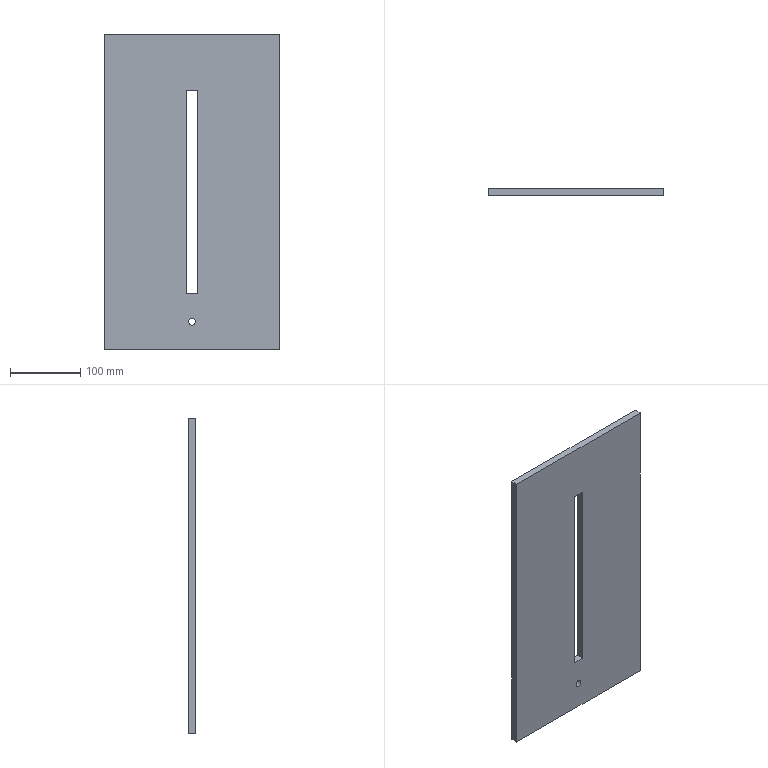Part | STEP file | tieqianjijia | 1 solid | 11 faces | box 250 x 10 x 450 mm | volume 1077815 mm3 | plane 10 | cylinder 1 | commonest cylinder face diameters 10 x1
STEP:
#1=CARTESIAN_POINT('',(0.,0.,0.));
#2=DIRECTION('',(0.,0.,1.));
#3=DIRECTION('',(1.,0.,0.));
#4=AXIS2_PLACEMENT_3D('',#1,#2,#3);
#5=CARTESIAN_POINT('',(0.,5.,-180.));
#6=VERTEX_POINT('',#5);
#7=CARTESIAN_POINT('',(0.,5.,-185.));
#8=DIRECTION('',(0.,1.,0.));
#9=DIRECTION('',(0.,0.,1.));
#10=AXIS2_PLACEMENT_3D('',#7,#8,#9);
#11=CIRCLE('',#10,5.);
#12=CARTESIAN_POINT('',(0.,5.,0.));
#13=DIRECTION('',(0.,1.,0.));
#14=DIRECTION('',(0.,0.,1.));
#15=AXIS2_PLACEMENT_3D('',#12,#13,#14);
#16=PLANE('',#15);
#17=CARTESIAN_POINT('',(-185.,0.));
#18=DIRECTION('',(1.,0.));
#19=AXIS2_PLACEMENT_2D('',#17,#18);
#20=CIRCLE('',#19,5.);
#21=(GEOMETRIC_REPRESENTATION_CONTEXT(2)PARAMETRIC_REPRESENTATION_CONTEXT()REPRESENTATION_CONTEXT('',''));
#22=DEFINITIONAL_REPRESENTATION('',(#20),#21);
#23=PCURVE('',#16,#22);
#24=CARTESIAN_POINT('',(0.,-5.,-185.));
#25=DIRECTION('',(0.,1.,0.));
#26=DIRECTION('',(0.,0.,1.));
#27=AXIS2_PLACEMENT_3D('',#24,#25,#26);
#28=CYLINDRICAL_SURFACE('',#27,5.);
#29=CARTESIAN_POINT('',(0.,10.));
#30=DIRECTION('',(1.,0.));
#31=VECTOR('',#30,1.);
#32=LINE('',#29,#31);
#33=(GEOMETRIC_REPRESENTATION_CONTEXT(2)PARAMETRIC_REPRESENTATION_CONTEXT()REPRESENTATION_CONTEXT('',''));
#34=DEFINITIONAL_REPRESENTATION('',(#32),#33);
#35=PCURVE('',#28,#34);
#36=SURFACE_CURVE('',#11,(#23,#35),.PCURVE_S1.);
#37=EDGE_CURVE('',#6,#6,#36,.T.);
#38=ORIENTED_EDGE('',*,*,#37,.F.);
#39=EDGE_LOOP('',(#38));
#40=FACE_BOUND('',#39,.T.);
#41=CARTESIAN_POINT('',(125.,5.,225.));
#42=VERTEX_POINT('',#41);
#43=CARTESIAN_POINT('',(125.,5.,-225.));
#44=VERTEX_POINT('',#43);
#45=CARTESIAN_POINT('',(125.,5.,-225.));
#46=DIRECTION('',(0.,0.,-1.));
#47=VECTOR('',#46,1.);
#48=LINE('',#45,#47);
#49=CARTESIAN_POINT('',(-225.,125.));
#50=DIRECTION('',(-1.,0.));
#51=VECTOR('',#50,1.);
#52=LINE('',#49,#51);
#53=(GEOMETRIC_REPRESENTATION_CONTEXT(2)PARAMETRIC_REPRESENTATION_CONTEXT()REPRESENTATION_CONTEXT('',''));
#54=DEFINITIONAL_REPRESENTATION('',(#52),#53);
#55=PCURVE('',#16,#54);
#56=CARTESIAN_POINT('',(125.,5.,-225.));
#57=DIRECTION('',(-1.,0.,0.));
#58=DIRECTION('',(0.,0.,1.));
#59=AXIS2_PLACEMENT_3D('',#56,#57,#58);
#60=PLANE('',#59);
#61=CARTESIAN_POINT('',(0.,0.));
#62=DIRECTION('',(-1.,0.));
#63=VECTOR('',#62,1.);
#64=LINE('',#61,#63);
#65=(GEOMETRIC_REPRESENTATION_CONTEXT(2)PARAMETRIC_REPRESENTATION_CONTEXT()REPRESENTATION_CONTEXT('',''));
#66=DEFINITIONAL_REPRESENTATION('',(#64),#65);
#67=PCURVE('',#60,#66);
#68=SURFACE_CURVE('',#48,(#55,#67),.PCURVE_S1.);
#69=EDGE_CURVE('',#42,#44,#68,.T.);
#70=ORIENTED_EDGE('',*,*,#69,.T.);
#71=CARTESIAN_POINT('',(-125.,5.,-225.));
#72=VERTEX_POINT('',#71);
#73=CARTESIAN_POINT('',(-125.,5.,-225.));
#74=DIRECTION('',(-1.,0.,0.));
#75=VECTOR('',#74,1.);
#76=LINE('',#73,#75);
#77=CARTESIAN_POINT('',(-225.,-125.));
#78=DIRECTION('',(0.,-1.));
#79=VECTOR('',#78,1.);
#80=LINE('',#77,#79);
#81=(GEOMETRIC_REPRESENTATION_CONTEXT(2)PARAMETRIC_REPRESENTATION_CONTEXT()REPRESENTATION_CONTEXT('',''));
#82=DEFINITIONAL_REPRESENTATION('',(#80),#81);
#83=PCURVE('',#16,#82);
#84=CARTESIAN_POINT('',(-125.,5.,-225.));
#85=DIRECTION('',(0.,0.,1.));
#86=DIRECTION('',(1.,0.,0.));
#87=AXIS2_PLACEMENT_3D('',#84,#85,#86);
#88=PLANE('',#87);
#89=CARTESIAN_POINT('',(0.,0.));
#90=DIRECTION('',(-1.,0.));
#91=VECTOR('',#90,1.);
#92=LINE('',#89,#91);
#93=(GEOMETRIC_REPRESENTATION_CONTEXT(2)PARAMETRIC_REPRESENTATION_CONTEXT()REPRESENTATION_CONTEXT('',''));
#94=DEFINITIONAL_REPRESENTATION('',(#92),#93);
#95=PCURVE('',#88,#94);
#96=SURFACE_CURVE('',#76,(#83,#95),.PCURVE_S1.);
#97=EDGE_CURVE('',#44,#72,#96,.T.);
#98=ORIENTED_EDGE('',*,*,#97,.T.);
#99=CARTESIAN_POINT('',(-125.,5.,225.));
#100=VERTEX_POINT('',#99);
#101=CARTESIAN_POINT('',(-125.,5.,-225.));
#102=DIRECTION('',(0.,0.,1.));
#103=VECTOR('',#102,1.);
#104=LINE('',#101,#103);
#105=CARTESIAN_POINT('',(-225.,-125.));
#106=DIRECTION('',(1.,0.));
#107=VECTOR('',#106,1.);
#108=LINE('',#105,#107);
#109=(GEOMETRIC_REPRESENTATION_CONTEXT(2)PARAMETRIC_REPRESENTATION_CONTEXT()REPRESENTATION_CONTEXT('',''));
#110=DEFINITIONAL_REPRESENTATION('',(#108),#109);
#111=PCURVE('',#16,#110);
#112=CARTESIAN_POINT('',(-125.,5.,-225.));
#113=DIRECTION('',(1.,0.,0.));
#114=DIRECTION('',(0.,0.,-1.));
#115=AXIS2_PLACEMENT_3D('',#112,#113,#114);
#116=PLANE('',#115);
#117=CARTESIAN_POINT('',(0.,0.));
#118=DIRECTION('',(-1.,0.));
#119=VECTOR('',#118,1.);
#120=LINE('',#117,#119);
#121=(GEOMETRIC_REPRESENTATION_CONTEXT(2)PARAMETRIC_REPRESENTATION_CONTEXT()REPRESENTATION_CONTEXT('',''));
#122=DEFINITIONAL_REPRESENTATION('',(#120),#121);
#123=PCURVE('',#116,#122);
#124=SURFACE_CURVE('',#104,(#111,#123),.PCURVE_S1.);
#125=EDGE_CURVE('',#72,#100,#124,.T.);
#126=ORIENTED_EDGE('',*,*,#125,.T.);
#127=CARTESIAN_POINT('',(-125.,5.,225.));
#128=DIRECTION('',(1.,0.,0.));
#129=VECTOR('',#128,1.);
#130=LINE('',#127,#129);
#131=CARTESIAN_POINT('',(225.,-125.));
#132=DIRECTION('',(0.,1.));
#133=VECTOR('',#132,1.);
#134=LINE('',#131,#133);
#135=(GEOMETRIC_REPRESENTATION_CONTEXT(2)PARAMETRIC_REPRESENTATION_CONTEXT()REPRESENTATION_CONTEXT('',''));
#136=DEFINITIONAL_REPRESENTATION('',(#134),#135);
#137=PCURVE('',#16,#136);
#138=CARTESIAN_POINT('',(-125.,5.,225.));
#139=DIRECTION('',(0.,0.,-1.));
#140=DIRECTION('',(-1.,0.,0.));
#141=AXIS2_PLACEMENT_3D('',#138,#139,#140);
#142=PLANE('',#141);
#143=CARTESIAN_POINT('',(0.,0.));
#144=DIRECTION('',(-1.,0.));
#145=VECTOR('',#144,1.);
#146=LINE('',#143,#145);
#147=(GEOMETRIC_REPRESENTATION_CONTEXT(2)PARAMETRIC_REPRESENTATION_CONTEXT()REPRESENTATION_CONTEXT('',''));
#148=DEFINITIONAL_REPRESENTATION('',(#146),#147);
#149=PCURVE('',#142,#148);
#150=SURFACE_CURVE('',#130,(#137,#149),.PCURVE_S1.);
#151=EDGE_CURVE('',#100,#42,#150,.T.);
#152=ORIENTED_EDGE('',*,*,#151,.T.);
#153=EDGE_LOOP('',(#70,#98,#126,#152));
#154=FACE_BOUND('',#153,.T.);
#155=CARTESIAN_POINT('',(8.,5.,-145.));
#156=VERTEX_POINT('',#155);
#157=CARTESIAN_POINT('',(-8.,5.,-145.));
#158=VERTEX_POINT('',#157);
#159=CARTESIAN_POINT('',(-8.,5.,-145.));
#160=DIRECTION('',(-1.,0.,0.));
#161=VECTOR('',#160,1.);
#162=LINE('',#159,#161);
#163=CARTESIAN_POINT('',(-145.,-8.));
#164=DIRECTION('',(0.,-1.));
#165=VECTOR('',#164,1.);
#166=LINE('',#163,#165);
#167=(GEOMETRIC_REPRESENTATION_CONTEXT(2)PARAMETRIC_REPRESENTATION_CONTEXT()REPRESENTATION_CONTEXT('',''));
#168=DEFINITIONAL_REPRESENTATION('',(#166),#167);
#169=PCURVE('',#16,#168);
#170=CARTESIAN_POINT('',(-8.,5.,-145.));
#171=DIRECTION('',(0.,0.,1.));
#172=DIRECTION('',(1.,0.,0.));
#173=AXIS2_PLACEMENT_3D('',#170,#171,#172);
#174=PLANE('',#173);
#175=CARTESIAN_POINT('',(0.,0.));
#176=DIRECTION('',(-1.,0.));
#177=VECTOR('',#176,1.);
#178=LINE('',#175,#177);
#179=(GEOMETRIC_REPRESENTATION_CONTEXT(2)PARAMETRIC_REPRESENTATION_CONTEXT()REPRESENTATION_CONTEXT('',''));
#180=DEFINITIONAL_REPRESENTATION('',(#178),#179);
#181=PCURVE('',#174,#180);
#182=SURFACE_CURVE('',#162,(#169,#181),.PCURVE_S1.);
#183=EDGE_CURVE('',#156,#158,#182,.T.);
#184=ORIENTED_EDGE('',*,*,#183,.F.);
#185=CARTESIAN_POINT('',(8.,5.,145.));
#186=VERTEX_POINT('',#185);
#187=CARTESIAN_POINT('',(8.,5.,-145.));
#188=DIRECTION('',(0.,0.,-1.));
#189=VECTOR('',#188,1.);
#190=LINE('',#187,#189);
#191=CARTESIAN_POINT('',(-145.,8.));
#192=DIRECTION('',(-1.,0.));
#193=VECTOR('',#192,1.);
#194=LINE('',#191,#193);
#195=(GEOMETRIC_REPRESENTATION_CONTEXT(2)PARAMETRIC_REPRESENTATION_CONTEXT()REPRESENTATION_CONTEXT('',''));
#196=DEFINITIONAL_REPRESENTATION('',(#194),#195);
#197=PCURVE('',#16,#196);
#198=CARTESIAN_POINT('',(8.,5.,-145.));
#199=DIRECTION('',(-1.,0.,0.));
#200=DIRECTION('',(0.,0.,1.));
#201=AXIS2_PLACEMENT_3D('',#198,#199,#200);
#202=PLANE('',#201);
#203=CARTESIAN_POINT('',(0.,0.));
#204=DIRECTION('',(-1.,0.));
#205=VECTOR('',#204,1.);
#206=LINE('',#203,#205);
#207=(GEOMETRIC_REPRESENTATION_CONTEXT(2)PARAMETRIC_REPRESENTATION_CONTEXT()REPRESENTATION_CONTEXT('',''));
#208=DEFINITIONAL_REPRESENTATION('',(#206),#207);
#209=PCURVE('',#202,#208);
#210=SURFACE_CURVE('',#190,(#197,#209),.PCURVE_S1.);
#211=EDGE_CURVE('',#186,#156,#210,.T.);
#212=ORIENTED_EDGE('',*,*,#211,.F.);
#213=CARTESIAN_POINT('',(-8.,5.,145.));
#214=VERTEX_POINT('',#213);
#215=CARTESIAN_POINT('',(-8.,5.,145.));
#216=DIRECTION('',(1.,0.,0.));
#217=VECTOR('',#216,1.);
#218=LINE('',#215,#217);
#219=CARTESIAN_POINT('',(145.,-8.));
#220=DIRECTION('',(0.,1.));
#221=VECTOR('',#220,1.);
#222=LINE('',#219,#221);
#223=(GEOMETRIC_REPRESENTATION_CONTEXT(2)PARAMETRIC_REPRESENTATION_CONTEXT()REPRESENTATION_CONTEXT('',''));
#224=DEFINITIONAL_REPRESENTATION('',(#222),#223);
#225=PCURVE('',#16,#224);
#226=CARTESIAN_POINT('',(-8.,5.,145.));
#227=DIRECTION('',(0.,0.,-1.));
#228=DIRECTION('',(-1.,0.,0.));
#229=AXIS2_PLACEMENT_3D('',#226,#227,#228);
#230=PLANE('',#229);
#231=CARTESIAN_POINT('',(0.,0.));
#232=DIRECTION('',(-1.,0.));
#233=VECTOR('',#232,1.);
#234=LINE('',#231,#233);
#235=(GEOMETRIC_REPRESENTATION_CONTEXT(2)PARAMETRIC_REPRESENTATION_CONTEXT()REPRESENTATION_CONTEXT('',''));
#236=DEFINITIONAL_REPRESENTATION('',(#234),#235);
#237=PCURVE('',#230,#236);
#238=SURFACE_CURVE('',#218,(#225,#237),.PCURVE_S1.);
#239=EDGE_CURVE('',#214,#186,#238,.T.);
#240=ORIENTED_EDGE('',*,*,#239,.F.);
#241=CARTESIAN_POINT('',(-8.,5.,-145.));
#242=DIRECTION('',(0.,0.,1.));
#243=VECTOR('',#242,1.);
#244=LINE('',#241,#243);
#245=CARTESIAN_POINT('',(-145.,-8.));
#246=DIRECTION('',(1.,0.));
#247=VECTOR('',#246,1.);
#248=LINE('',#245,#247);
#249=(GEOMETRIC_REPRESENTATION_CONTEXT(2)PARAMETRIC_REPRESENTATION_CONTEXT()REPRESENTATION_CONTEXT('',''));
#250=DEFINITIONAL_REPRESENTATION('',(#248),#249);
#251=PCURVE('',#16,#250);
#252=CARTESIAN_POINT('',(-8.,5.,-145.));
#253=DIRECTION('',(1.,0.,0.));
#254=DIRECTION('',(0.,0.,-1.));
#255=AXIS2_PLACEMENT_3D('',#252,#253,#254);
#256=PLANE('',#255);
#257=CARTESIAN_POINT('',(0.,0.));
#258=DIRECTION('',(-1.,0.));
#259=VECTOR('',#258,1.);
#260=LINE('',#257,#259);
#261=(GEOMETRIC_REPRESENTATION_CONTEXT(2)PARAMETRIC_REPRESENTATION_CONTEXT()REPRESENTATION_CONTEXT('',''));
#262=DEFINITIONAL_REPRESENTATION('',(#260),#261);
#263=PCURVE('',#256,#262);
#264=SURFACE_CURVE('',#244,(#251,#263),.PCURVE_S1.);
#265=EDGE_CURVE('',#158,#214,#264,.T.);
#266=ORIENTED_EDGE('',*,*,#265,.F.);
#267=EDGE_LOOP('',(#184,#212,#240,#266));
#268=FACE_BOUND('',#267,.T.);
#269=ADVANCED_FACE('',(#40,#154,#268),#16,.T.);
#270=CARTESIAN_POINT('',(0.,-5.,-180.));
#271=VERTEX_POINT('',#270);
#272=CARTESIAN_POINT('',(0.,-5.,-185.));
#273=DIRECTION('',(0.,1.,0.));
#274=DIRECTION('',(0.,0.,1.));
#275=AXIS2_PLACEMENT_3D('',#272,#273,#274);
#276=CIRCLE('',#275,5.);
#277=CARTESIAN_POINT('',(0.,-5.,0.));
#278=DIRECTION('',(0.,1.,0.));
#279=DIRECTION('',(0.,0.,1.));
#280=AXIS2_PLACEMENT_3D('',#277,#278,#279);
#281=PLANE('',#280);
#282=CARTESIAN_POINT('',(-185.,0.));
#283=DIRECTION('',(1.,0.));
#284=AXIS2_PLACEMENT_2D('',#282,#283);
#285=CIRCLE('',#284,5.);
#286=(GEOMETRIC_REPRESENTATION_CONTEXT(2)PARAMETRIC_REPRESENTATION_CONTEXT()REPRESENTATION_CONTEXT('',''));
#287=DEFINITIONAL_REPRESENTATION('',(#285),#286);
#288=PCURVE('',#281,#287);
#289=CARTESIAN_POINT('',(0.,0.));
#290=DIRECTION('',(1.,0.));
#291=VECTOR('',#290,1.);
#292=LINE('',#289,#291);
#293=(GEOMETRIC_REPRESENTATION_CONTEXT(2)PARAMETRIC_REPRESENTATION_CONTEXT()REPRESENTATION_CONTEXT('',''));
#294=DEFINITIONAL_REPRESENTATION('',(#292),#293);
#295=PCURVE('',#28,#294);
#296=SURFACE_CURVE('',#276,(#288,#295),.PCURVE_S1.);
#297=EDGE_CURVE('',#271,#271,#296,.T.);
#298=ORIENTED_EDGE('',*,*,#297,.T.);
#299=EDGE_LOOP('',(#298));
#300=FACE_BOUND('',#299,.T.);
#301=CARTESIAN_POINT('',(125.,-5.,225.));
#302=VERTEX_POINT('',#301);
#303=CARTESIAN_POINT('',(125.,-5.,-225.));
#304=VERTEX_POINT('',#303);
#305=CARTESIAN_POINT('',(125.,-5.,-225.));
#306=DIRECTION('',(0.,0.,-1.));
#307=VECTOR('',#306,1.);
#308=LINE('',#305,#307);
#309=CARTESIAN_POINT('',(-225.,125.));
#310=DIRECTION('',(-1.,0.));
#311=VECTOR('',#310,1.);
#312=LINE('',#309,#311);
#313=(GEOMETRIC_REPRESENTATION_CONTEXT(2)PARAMETRIC_REPRESENTATION_CONTEXT()REPRESENTATION_CONTEXT('',''));
#314=DEFINITIONAL_REPRESENTATION('',(#312),#313);
#315=PCURVE('',#281,#314);
#316=CARTESIAN_POINT('',(0.,-10.));
#317=DIRECTION('',(-1.,0.));
#318=VECTOR('',#317,1.);
#319=LINE('',#316,#318);
#320=(GEOMETRIC_REPRESENTATION_CONTEXT(2)PARAMETRIC_REPRESENTATION_CONTEXT()REPRESENTATION_CONTEXT('',''));
#321=DEFINITIONAL_REPRESENTATION('',(#319),#320);
#322=PCURVE('',#60,#321);
#323=SURFACE_CURVE('',#308,(#315,#322),.PCURVE_S1.);
#324=EDGE_CURVE('',#302,#304,#323,.T.);
#325=ORIENTED_EDGE('',*,*,#324,.F.);
#326=CARTESIAN_POINT('',(-125.,-5.,225.));
#327=VERTEX_POINT('',#326);
#328=CARTESIAN_POINT('',(-125.,-5.,225.));
#329=DIRECTION('',(1.,0.,0.));
#330=VECTOR('',#329,1.);
#331=LINE('',#328,#330);
#332=CARTESIAN_POINT('',(225.,-125.));
#333=DIRECTION('',(0.,1.));
#334=VECTOR('',#333,1.);
#335=LINE('',#332,#334);
#336=(GEOMETRIC_REPRESENTATION_CONTEXT(2)PARAMETRIC_REPRESENTATION_CONTEXT()REPRESENTATION_CONTEXT('',''));
#337=DEFINITIONAL_REPRESENTATION('',(#335),#336);
#338=PCURVE('',#281,#337);
#339=CARTESIAN_POINT('',(0.,-10.));
#340=DIRECTION('',(-1.,0.));
#341=VECTOR('',#340,1.);
#342=LINE('',#339,#341);
#343=(GEOMETRIC_REPRESENTATION_CONTEXT(2)PARAMETRIC_REPRESENTATION_CONTEXT()REPRESENTATION_CONTEXT('',''));
#344=DEFINITIONAL_REPRESENTATION('',(#342),#343);
#345=PCURVE('',#142,#344);
#346=SURFACE_CURVE('',#331,(#338,#345),.PCURVE_S1.);
#347=EDGE_CURVE('',#327,#302,#346,.T.);
#348=ORIENTED_EDGE('',*,*,#347,.F.);
#349=CARTESIAN_POINT('',(-125.,-5.,-225.));
#350=VERTEX_POINT('',#349);
#351=CARTESIAN_POINT('',(-125.,-5.,-225.));
#352=DIRECTION('',(0.,0.,1.));
#353=VECTOR('',#352,1.);
#354=LINE('',#351,#353);
#355=CARTESIAN_POINT('',(-225.,-125.));
#356=DIRECTION('',(1.,0.));
#357=VECTOR('',#356,1.);
#358=LINE('',#355,#357);
#359=(GEOMETRIC_REPRESENTATION_CONTEXT(2)PARAMETRIC_REPRESENTATION_CONTEXT()REPRESENTATION_CONTEXT('',''));
#360=DEFINITIONAL_REPRESENTATION('',(#358),#359);
#361=PCURVE('',#281,#360);
#362=CARTESIAN_POINT('',(0.,-10.));
#363=DIRECTION('',(-1.,0.));
#364=VECTOR('',#363,1.);
#365=LINE('',#362,#364);
#366=(GEOMETRIC_REPRESENTATION_CONTEXT(2)PARAMETRIC_REPRESENTATION_CONTEXT()REPRESENTATION_CONTEXT('',''));
#367=DEFINITIONAL_REPRESENTATION('',(#365),#366);
#368=PCURVE('',#116,#367);
#369=SURFACE_CURVE('',#354,(#361,#368),.PCURVE_S1.);
#370=EDGE_CURVE('',#350,#327,#369,.T.);
#371=ORIENTED_EDGE('',*,*,#370,.F.);
#372=CARTESIAN_POINT('',(-125.,-5.,-225.));
#373=DIRECTION('',(-1.,0.,0.));
#374=VECTOR('',#373,1.);
#375=LINE('',#372,#374);
#376=CARTESIAN_POINT('',(-225.,-125.));
#377=DIRECTION('',(0.,-1.));
#378=VECTOR('',#377,1.);
#379=LINE('',#376,#378);
#380=(GEOMETRIC_REPRESENTATION_CONTEXT(2)PARAMETRIC_REPRESENTATION_CONTEXT()REPRESENTATION_CONTEXT('',''));
#381=DEFINITIONAL_REPRESENTATION('',(#379),#380);
#382=PCURVE('',#281,#381);
#383=CARTESIAN_POINT('',(0.,-10.));
#384=DIRECTION('',(-1.,0.));
#385=VECTOR('',#384,1.);
#386=LINE('',#383,#385);
#387=(GEOMETRIC_REPRESENTATION_CONTEXT(2)PARAMETRIC_REPRESENTATION_CONTEXT()REPRESENTATION_CONTEXT('',''));
#388=DEFINITIONAL_REPRESENTATION('',(#386),#387);
#389=PCURVE('',#88,#388);
#390=SURFACE_CURVE('',#375,(#382,#389),.PCURVE_S1.);
#391=EDGE_CURVE('',#304,#350,#390,.T.);
#392=ORIENTED_EDGE('',*,*,#391,.F.);
#393=EDGE_LOOP('',(#325,#348,#371,#392));
#394=FACE_BOUND('',#393,.T.);
#395=CARTESIAN_POINT('',(8.,-5.,145.));
#396=VERTEX_POINT('',#395);
#397=CARTESIAN_POINT('',(8.,-5.,-145.));
#398=VERTEX_POINT('',#397);
#399=CARTESIAN_POINT('',(8.,-5.,-145.));
#400=DIRECTION('',(0.,0.,-1.));
#401=VECTOR('',#400,1.);
#402=LINE('',#399,#401);
#403=CARTESIAN_POINT('',(-145.,8.));
#404=DIRECTION('',(-1.,0.));
#405=VECTOR('',#404,1.);
#406=LINE('',#403,#405);
#407=(GEOMETRIC_REPRESENTATION_CONTEXT(2)PARAMETRIC_REPRESENTATION_CONTEXT()REPRESENTATION_CONTEXT('',''));
#408=DEFINITIONAL_REPRESENTATION('',(#406),#407);
#409=PCURVE('',#281,#408);
#410=CARTESIAN_POINT('',(0.,-10.));
#411=DIRECTION('',(-1.,0.));
#412=VECTOR('',#411,1.);
#413=LINE('',#410,#412);
#414=(GEOMETRIC_REPRESENTATION_CONTEXT(2)PARAMETRIC_REPRESENTATION_CONTEXT()REPRESENTATION_CONTEXT('',''));
#415=DEFINITIONAL_REPRESENTATION('',(#413),#414);
#416=PCURVE('',#202,#415);
#417=SURFACE_CURVE('',#402,(#409,#416),.PCURVE_S1.);
#418=EDGE_CURVE('',#396,#398,#417,.T.);
#419=ORIENTED_EDGE('',*,*,#418,.T.);
#420=CARTESIAN_POINT('',(-8.,-5.,-145.));
#421=VERTEX_POINT('',#420);
#422=CARTESIAN_POINT('',(-8.,-5.,-145.));
#423=DIRECTION('',(-1.,0.,0.));
#424=VECTOR('',#423,1.);
#425=LINE('',#422,#424);
#426=CARTESIAN_POINT('',(-145.,-8.));
#427=DIRECTION('',(0.,-1.));
#428=VECTOR('',#427,1.);
#429=LINE('',#426,#428);
#430=(GEOMETRIC_REPRESENTATION_CONTEXT(2)PARAMETRIC_REPRESENTATION_CONTEXT()REPRESENTATION_CONTEXT('',''));
#431=DEFINITIONAL_REPRESENTATION('',(#429),#430);
#432=PCURVE('',#281,#431);
#433=CARTESIAN_POINT('',(0.,-10.));
#434=DIRECTION('',(-1.,0.));
#435=VECTOR('',#434,1.);
#436=LINE('',#433,#435);
#437=(GEOMETRIC_REPRESENTATION_CONTEXT(2)PARAMETRIC_REPRESENTATION_CONTEXT()REPRESENTATION_CONTEXT('',''));
#438=DEFINITIONAL_REPRESENTATION('',(#436),#437);
#439=PCURVE('',#174,#438);
#440=SURFACE_CURVE('',#425,(#432,#439),.PCURVE_S1.);
#441=EDGE_CURVE('',#398,#421,#440,.T.);
#442=ORIENTED_EDGE('',*,*,#441,.T.);
#443=CARTESIAN_POINT('',(-8.,-5.,145.));
#444=VERTEX_POINT('',#443);
#445=CARTESIAN_POINT('',(-8.,-5.,-145.));
#446=DIRECTION('',(0.,0.,1.));
#447=VECTOR('',#446,1.);
#448=LINE('',#445,#447);
#449=CARTESIAN_POINT('',(-145.,-8.));
#450=DIRECTION('',(1.,0.));
#451=VECTOR('',#450,1.);
#452=LINE('',#449,#451);
#453=(GEOMETRIC_REPRESENTATION_CONTEXT(2)PARAMETRIC_REPRESENTATION_CONTEXT()REPRESENTATION_CONTEXT('',''));
#454=DEFINITIONAL_REPRESENTATION('',(#452),#453);
#455=PCURVE('',#281,#454);
#456=CARTESIAN_POINT('',(0.,-10.));
#457=DIRECTION('',(-1.,0.));
#458=VECTOR('',#457,1.);
#459=LINE('',#456,#458);
#460=(GEOMETRIC_REPRESENTATION_CONTEXT(2)PARAMETRIC_REPRESENTATION_CONTEXT()REPRESENTATION_CONTEXT('',''));
#461=DEFINITIONAL_REPRESENTATION('',(#459),#460);
#462=PCURVE('',#256,#461);
#463=SURFACE_CURVE('',#448,(#455,#462),.PCURVE_S1.);
#464=EDGE_CURVE('',#421,#444,#463,.T.);
#465=ORIENTED_EDGE('',*,*,#464,.T.);
#466=CARTESIAN_POINT('',(-8.,-5.,145.));
#467=DIRECTION('',(1.,0.,0.));
#468=VECTOR('',#467,1.);
#469=LINE('',#466,#468);
#470=CARTESIAN_POINT('',(145.,-8.));
#471=DIRECTION('',(0.,1.));
#472=VECTOR('',#471,1.);
#473=LINE('',#470,#472);
#474=(GEOMETRIC_REPRESENTATION_CONTEXT(2)PARAMETRIC_REPRESENTATION_CONTEXT()REPRESENTATION_CONTEXT('',''));
#475=DEFINITIONAL_REPRESENTATION('',(#473),#474);
#476=PCURVE('',#281,#475);
#477=CARTESIAN_POINT('',(0.,-10.));
#478=DIRECTION('',(-1.,0.));
#479=VECTOR('',#478,1.);
#480=LINE('',#477,#479);
#481=(GEOMETRIC_REPRESENTATION_CONTEXT(2)PARAMETRIC_REPRESENTATION_CONTEXT()REPRESENTATION_CONTEXT('',''));
#482=DEFINITIONAL_REPRESENTATION('',(#480),#481);
#483=PCURVE('',#230,#482);
#484=SURFACE_CURVE('',#469,(#476,#483),.PCURVE_S1.);
#485=EDGE_CURVE('',#444,#396,#484,.T.);
#486=ORIENTED_EDGE('',*,*,#485,.T.);
#487=EDGE_LOOP('',(#419,#442,#465,#486));
#488=FACE_BOUND('',#487,.T.);
#489=ADVANCED_FACE('',(#300,#394,#488),#281,.F.);
#490=ORIENTED_EDGE('',*,*,#324,.T.);
#491=CARTESIAN_POINT('',(125.,5.,-225.));
#492=DIRECTION('',(0.,-1.,0.));
#493=VECTOR('',#492,1.);
#494=LINE('',#491,#493);
#495=CARTESIAN_POINT('',(0.,0.));
#496=DIRECTION('',(0.,-1.));
#497=VECTOR('',#496,1.);
#498=LINE('',#495,#497);
#499=(GEOMETRIC_REPRESENTATION_CONTEXT(2)PARAMETRIC_REPRESENTATION_CONTEXT()REPRESENTATION_CONTEXT('',''));
#500=DEFINITIONAL_REPRESENTATION('',(#498),#499);
#501=PCURVE('',#60,#500);
#502=CARTESIAN_POINT('',(250.,0.));
#503=DIRECTION('',(0.,-1.));
#504=VECTOR('',#503,1.);
#505=LINE('',#502,#504);
#506=(GEOMETRIC_REPRESENTATION_CONTEXT(2)PARAMETRIC_REPRESENTATION_CONTEXT()REPRESENTATION_CONTEXT('',''));
#507=DEFINITIONAL_REPRESENTATION('',(#505),#506);
#508=PCURVE('',#88,#507);
#509=SURFACE_CURVE('',#494,(#501,#508),.PCURVE_S1.);
#510=EDGE_CURVE('',#44,#304,#509,.T.);
#511=ORIENTED_EDGE('',*,*,#510,.F.);
#512=ORIENTED_EDGE('',*,*,#69,.F.);
#513=CARTESIAN_POINT('',(125.,5.,225.));
#514=DIRECTION('',(0.,-1.,0.));
#515=VECTOR('',#514,1.);
#516=LINE('',#513,#515);
#517=CARTESIAN_POINT('',(450.,0.));
#518=DIRECTION('',(0.,-1.));
#519=VECTOR('',#518,1.);
#520=LINE('',#517,#519);
#521=(GEOMETRIC_REPRESENTATION_CONTEXT(2)PARAMETRIC_REPRESENTATION_CONTEXT()REPRESENTATION_CONTEXT('',''));
#522=DEFINITIONAL_REPRESENTATION('',(#520),#521);
#523=PCURVE('',#60,#522);
#524=CARTESIAN_POINT('',(-250.,0.));
#525=DIRECTION('',(0.,-1.));
#526=VECTOR('',#525,1.);
#527=LINE('',#524,#526);
#528=(GEOMETRIC_REPRESENTATION_CONTEXT(2)PARAMETRIC_REPRESENTATION_CONTEXT()REPRESENTATION_CONTEXT('',''));
#529=DEFINITIONAL_REPRESENTATION('',(#527),#528);
#530=PCURVE('',#142,#529);
#531=SURFACE_CURVE('',#516,(#523,#530),.PCURVE_S1.);
#532=EDGE_CURVE('',#42,#302,#531,.T.);
#533=ORIENTED_EDGE('',*,*,#532,.T.);
#534=EDGE_LOOP('',(#490,#511,#512,#533));
#535=FACE_BOUND('',#534,.T.);
#536=ADVANCED_FACE('',(#535),#60,.F.);
#537=ORIENTED_EDGE('',*,*,#391,.T.);
#538=CARTESIAN_POINT('',(-125.,5.,-225.));
#539=DIRECTION('',(0.,-1.,0.));
#540=VECTOR('',#539,1.);
#541=LINE('',#538,#540);
#542=CARTESIAN_POINT('',(0.,0.));
#543=DIRECTION('',(0.,-1.));
#544=VECTOR('',#543,1.);
#545=LINE('',#542,#544);
#546=(GEOMETRIC_REPRESENTATION_CONTEXT(2)PARAMETRIC_REPRESENTATION_CONTEXT()REPRESENTATION_CONTEXT('',''));
#547=DEFINITIONAL_REPRESENTATION('',(#545),#546);
#548=PCURVE('',#88,#547);
#549=CARTESIAN_POINT('',(0.,0.));
#550=DIRECTION('',(0.,-1.));
#551=VECTOR('',#550,1.);
#552=LINE('',#549,#551);
#553=(GEOMETRIC_REPRESENTATION_CONTEXT(2)PARAMETRIC_REPRESENTATION_CONTEXT()REPRESENTATION_CONTEXT('',''));
#554=DEFINITIONAL_REPRESENTATION('',(#552),#553);
#555=PCURVE('',#116,#554);
#556=SURFACE_CURVE('',#541,(#548,#555),.PCURVE_S1.);
#557=EDGE_CURVE('',#72,#350,#556,.T.);
#558=ORIENTED_EDGE('',*,*,#557,.F.);
#559=ORIENTED_EDGE('',*,*,#97,.F.);
#560=ORIENTED_EDGE('',*,*,#510,.T.);
#561=EDGE_LOOP('',(#537,#558,#559,#560));
#562=FACE_BOUND('',#561,.T.);
#563=ADVANCED_FACE('',(#562),#88,.F.);
#564=ORIENTED_EDGE('',*,*,#370,.T.);
#565=CARTESIAN_POINT('',(-125.,5.,225.));
#566=DIRECTION('',(0.,-1.,0.));
#567=VECTOR('',#566,1.);
#568=LINE('',#565,#567);
#569=CARTESIAN_POINT('',(-450.,0.));
#570=DIRECTION('',(0.,-1.));
#571=VECTOR('',#570,1.);
#572=LINE('',#569,#571);
#573=(GEOMETRIC_REPRESENTATION_CONTEXT(2)PARAMETRIC_REPRESENTATION_CONTEXT()REPRESENTATION_CONTEXT('',''));
#574=DEFINITIONAL_REPRESENTATION('',(#572),#573);
#575=PCURVE('',#116,#574);
#576=CARTESIAN_POINT('',(0.,0.));
#577=DIRECTION('',(0.,-1.));
#578=VECTOR('',#577,1.);
#579=LINE('',#576,#578);
#580=(GEOMETRIC_REPRESENTATION_CONTEXT(2)PARAMETRIC_REPRESENTATION_CONTEXT()REPRESENTATION_CONTEXT('',''));
#581=DEFINITIONAL_REPRESENTATION('',(#579),#580);
#582=PCURVE('',#142,#581);
#583=SURFACE_CURVE('',#568,(#575,#582),.PCURVE_S1.);
#584=EDGE_CURVE('',#100,#327,#583,.T.);
#585=ORIENTED_EDGE('',*,*,#584,.F.);
#586=ORIENTED_EDGE('',*,*,#125,.F.);
#587=ORIENTED_EDGE('',*,*,#557,.T.);
#588=EDGE_LOOP('',(#564,#585,#586,#587));
#589=FACE_BOUND('',#588,.T.);
#590=ADVANCED_FACE('',(#589),#116,.F.);
#591=ORIENTED_EDGE('',*,*,#347,.T.);
#592=ORIENTED_EDGE('',*,*,#532,.F.);
#593=ORIENTED_EDGE('',*,*,#151,.F.);
#594=ORIENTED_EDGE('',*,*,#584,.T.);
#595=EDGE_LOOP('',(#591,#592,#593,#594));
#596=FACE_BOUND('',#595,.T.);
#597=ADVANCED_FACE('',(#596),#142,.F.);
#598=ORIENTED_EDGE('',*,*,#418,.F.);
#599=CARTESIAN_POINT('',(8.,5.,145.));
#600=DIRECTION('',(0.,-1.,0.));
#601=VECTOR('',#600,1.);
#602=LINE('',#599,#601);
#603=CARTESIAN_POINT('',(290.,0.));
#604=DIRECTION('',(0.,-1.));
#605=VECTOR('',#604,1.);
#606=LINE('',#603,#605);
#607=(GEOMETRIC_REPRESENTATION_CONTEXT(2)PARAMETRIC_REPRESENTATION_CONTEXT()REPRESENTATION_CONTEXT('',''));
#608=DEFINITIONAL_REPRESENTATION('',(#606),#607);
#609=PCURVE('',#202,#608);
#610=CARTESIAN_POINT('',(-16.,0.));
#611=DIRECTION('',(0.,-1.));
#612=VECTOR('',#611,1.);
#613=LINE('',#610,#612);
#614=(GEOMETRIC_REPRESENTATION_CONTEXT(2)PARAMETRIC_REPRESENTATION_CONTEXT()REPRESENTATION_CONTEXT('',''));
#615=DEFINITIONAL_REPRESENTATION('',(#613),#614);
#616=PCURVE('',#230,#615);
#617=SURFACE_CURVE('',#602,(#609,#616),.PCURVE_S1.);
#618=EDGE_CURVE('',#186,#396,#617,.T.);
#619=ORIENTED_EDGE('',*,*,#618,.F.);
#620=ORIENTED_EDGE('',*,*,#211,.T.);
#621=CARTESIAN_POINT('',(8.,5.,-145.));
#622=DIRECTION('',(0.,-1.,0.));
#623=VECTOR('',#622,1.);
#624=LINE('',#621,#623);
#625=CARTESIAN_POINT('',(0.,0.));
#626=DIRECTION('',(0.,-1.));
#627=VECTOR('',#626,1.);
#628=LINE('',#625,#627);
#629=(GEOMETRIC_REPRESENTATION_CONTEXT(2)PARAMETRIC_REPRESENTATION_CONTEXT()REPRESENTATION_CONTEXT('',''));
#630=DEFINITIONAL_REPRESENTATION('',(#628),#629);
#631=PCURVE('',#202,#630);
#632=CARTESIAN_POINT('',(16.,0.));
#633=DIRECTION('',(0.,-1.));
#634=VECTOR('',#633,1.);
#635=LINE('',#632,#634);
#636=(GEOMETRIC_REPRESENTATION_CONTEXT(2)PARAMETRIC_REPRESENTATION_CONTEXT()REPRESENTATION_CONTEXT('',''));
#637=DEFINITIONAL_REPRESENTATION('',(#635),#636);
#638=PCURVE('',#174,#637);
#639=SURFACE_CURVE('',#624,(#631,#638),.PCURVE_S1.);
#640=EDGE_CURVE('',#156,#398,#639,.T.);
#641=ORIENTED_EDGE('',*,*,#640,.T.);
#642=EDGE_LOOP('',(#598,#619,#620,#641));
#643=FACE_BOUND('',#642,.T.);
#644=ADVANCED_FACE('',(#643),#202,.T.);
#645=ORIENTED_EDGE('',*,*,#441,.F.);
#646=ORIENTED_EDGE('',*,*,#640,.F.);
#647=ORIENTED_EDGE('',*,*,#183,.T.);
#648=CARTESIAN_POINT('',(-8.,5.,-145.));
#649=DIRECTION('',(0.,-1.,0.));
#650=VECTOR('',#649,1.);
#651=LINE('',#648,#650);
#652=CARTESIAN_POINT('',(0.,0.));
#653=DIRECTION('',(0.,-1.));
#654=VECTOR('',#653,1.);
#655=LINE('',#652,#654);
#656=(GEOMETRIC_REPRESENTATION_CONTEXT(2)PARAMETRIC_REPRESENTATION_CONTEXT()REPRESENTATION_CONTEXT('',''));
#657=DEFINITIONAL_REPRESENTATION('',(#655),#656);
#658=PCURVE('',#174,#657);
#659=CARTESIAN_POINT('',(0.,0.));
#660=DIRECTION('',(0.,-1.));
#661=VECTOR('',#660,1.);
#662=LINE('',#659,#661);
#663=(GEOMETRIC_REPRESENTATION_CONTEXT(2)PARAMETRIC_REPRESENTATION_CONTEXT()REPRESENTATION_CONTEXT('',''));
#664=DEFINITIONAL_REPRESENTATION('',(#662),#663);
#665=PCURVE('',#256,#664);
#666=SURFACE_CURVE('',#651,(#658,#665),.PCURVE_S1.);
#667=EDGE_CURVE('',#158,#421,#666,.T.);
#668=ORIENTED_EDGE('',*,*,#667,.T.);
#669=EDGE_LOOP('',(#645,#646,#647,#668));
#670=FACE_BOUND('',#669,.T.);
#671=ADVANCED_FACE('',(#670),#174,.T.);
#672=ORIENTED_EDGE('',*,*,#464,.F.);
#673=ORIENTED_EDGE('',*,*,#667,.F.);
#674=ORIENTED_EDGE('',*,*,#265,.T.);
#675=CARTESIAN_POINT('',(-8.,5.,145.));
#676=DIRECTION('',(0.,-1.,0.));
#677=VECTOR('',#676,1.);
#678=LINE('',#675,#677);
#679=CARTESIAN_POINT('',(-290.,0.));
#680=DIRECTION('',(0.,-1.));
#681=VECTOR('',#680,1.);
#682=LINE('',#679,#681);
#683=(GEOMETRIC_REPRESENTATION_CONTEXT(2)PARAMETRIC_REPRESENTATION_CONTEXT()REPRESENTATION_CONTEXT('',''));
#684=DEFINITIONAL_REPRESENTATION('',(#682),#683);
#685=PCURVE('',#256,#684);
#686=CARTESIAN_POINT('',(0.,0.));
#687=DIRECTION('',(0.,-1.));
#688=VECTOR('',#687,1.);
#689=LINE('',#686,#688);
#690=(GEOMETRIC_REPRESENTATION_CONTEXT(2)PARAMETRIC_REPRESENTATION_CONTEXT()REPRESENTATION_CONTEXT('',''));
#691=DEFINITIONAL_REPRESENTATION('',(#689),#690);
#692=PCURVE('',#230,#691);
#693=SURFACE_CURVE('',#678,(#685,#692),.PCURVE_S1.);
#694=EDGE_CURVE('',#214,#444,#693,.T.);
#695=ORIENTED_EDGE('',*,*,#694,.T.);
#696=EDGE_LOOP('',(#672,#673,#674,#695));
#697=FACE_BOUND('',#696,.T.);
#698=ADVANCED_FACE('',(#697),#256,.T.);
#699=ORIENTED_EDGE('',*,*,#485,.F.);
#700=ORIENTED_EDGE('',*,*,#694,.F.);
#701=ORIENTED_EDGE('',*,*,#239,.T.);
#702=ORIENTED_EDGE('',*,*,#618,.T.);
#703=EDGE_LOOP('',(#699,#700,#701,#702));
#704=FACE_BOUND('',#703,.T.);
#705=ADVANCED_FACE('',(#704),#230,.T.);
#706=ORIENTED_EDGE('',*,*,#297,.T.);
#707=CARTESIAN_POINT('',(0.,-5.,-180.));
#708=CARTESIAN_POINT('',(0.,5.,-180.));
#709=B_SPLINE_CURVE_WITH_KNOTS('',1,(#707,#708),.UNSPECIFIED.,.F.,.F.,(2,2),(0.,10.),.PIECEWISE_BEZIER_KNOTS.);
#710=CARTESIAN_POINT('',(6.283,0.));
#711=DIRECTION('',(0.,1.));
#712=VECTOR('',#711,1.);
#713=LINE('',#710,#712);
#714=(GEOMETRIC_REPRESENTATION_CONTEXT(2)PARAMETRIC_REPRESENTATION_CONTEXT()REPRESENTATION_CONTEXT('',''));
#715=DEFINITIONAL_REPRESENTATION('',(#713),#714);
#716=PCURVE('',#28,#715);
#717=CARTESIAN_POINT('',(0.,0.));
#718=DIRECTION('',(0.,1.));
#719=VECTOR('',#718,1.);
#720=LINE('',#717,#719);
#721=(GEOMETRIC_REPRESENTATION_CONTEXT(2)PARAMETRIC_REPRESENTATION_CONTEXT()REPRESENTATION_CONTEXT('',''));
#722=DEFINITIONAL_REPRESENTATION('',(#720),#721);
#723=PCURVE('',#28,#722);
#724=SEAM_CURVE('',#709,(#716,#723),.PCURVE_S1.);
#725=EDGE_CURVE('',#271,#6,#724,.T.);
#726=ORIENTED_EDGE('',*,*,#725,.T.);
#727=ORIENTED_EDGE('',*,*,#37,.F.);
#728=ORIENTED_EDGE('',*,*,#725,.F.);
#729=EDGE_LOOP('',(#706,#726,#727,#728));
#730=FACE_BOUND('',#729,.F.);
#731=ADVANCED_FACE('',(#730),#28,.F.);
#732=CLOSED_SHELL('',(#269,#489,#536,#563,#590,#597,#644,#671,#698,#705,#731));
#733=MANIFOLD_SOLID_BREP('',#732);
#734=(LENGTH_UNIT()NAMED_UNIT(*)SI_UNIT(.MILLI.,.METRE.));
#735=UNCERTAINTY_MEASURE_WITH_UNIT(LENGTH_MEASURE(0.000001),#734,'','');
#736=(NAMED_UNIT(*)PLANE_ANGLE_UNIT()SI_UNIT($,.RADIAN.));
#737=(NAMED_UNIT(*)SI_UNIT($,.STERADIAN.)SOLID_ANGLE_UNIT());
#738=(GEOMETRIC_REPRESENTATION_CONTEXT(3)GLOBAL_UNCERTAINTY_ASSIGNED_CONTEXT((#735))GLOBAL_UNIT_ASSIGNED_CONTEXT((#734,#736,#737))REPRESENTATION_CONTEXT('',''));
#739=ADVANCED_BREP_SHAPE_REPRESENTATION('',(#4,#733),#738);